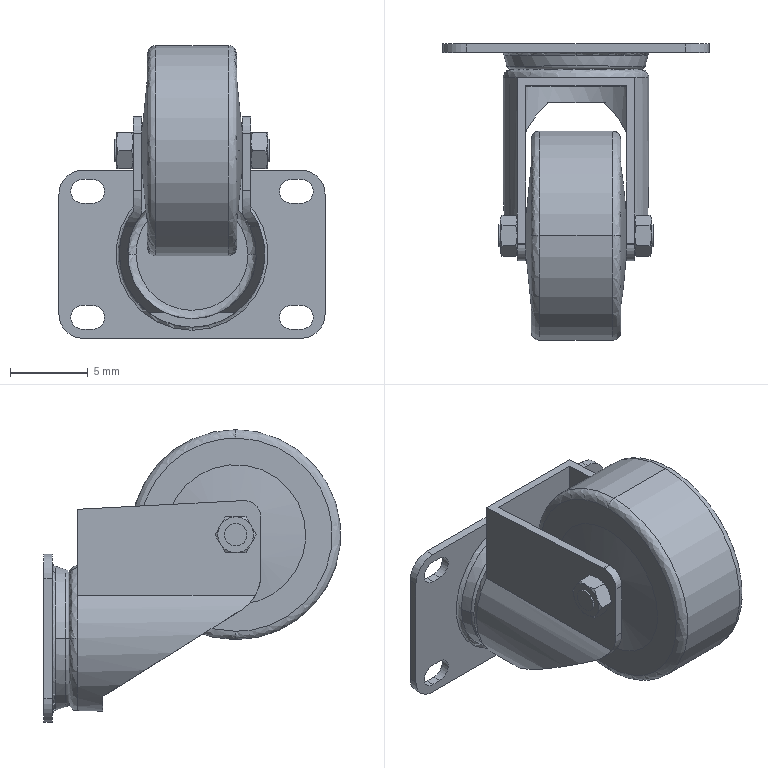Part | SolidWorks | features ICE 4, BaseBody 2, Fillet 2, Extrusion 1, Revolution 1, Scale 1 | 3 solids | 130 faces | box 17.1 x 19.08 x 18.81 mm | volume 1198 mm3 | plane 51 | cylinder 38 | cone 26 | spline 11 | torus 4 | commonest cylinder face diameters 1.53 x12 1.44 x8 2.16 x4 2.295 x4 3.06 x4 5.4 x2